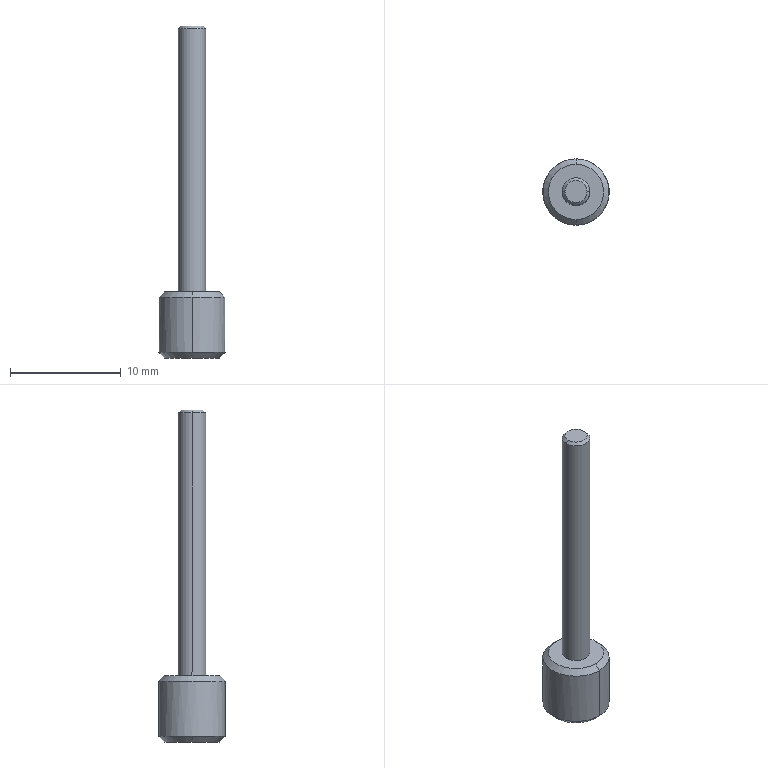Part | SolidWorks | features BaseBody 1 | 1 solid | 13 faces | box 6 x 6 x 30 mm | volume 282.776 mm3 | cone 6 | cylinder 4 | plane 3 | commonest cylinder face diameters 2.5 x2 6 x2
STEP:
#1=CARTESIAN_POINT('',(-45.25,9.997,38.261));
#2=VERTEX_POINT('',#1);
#3=CARTESIAN_POINT('',(-42.75,9.997,38.261));
#4=VERTEX_POINT('',#3);
#5=CARTESIAN_POINT('',(-44.,9.997,38.261));
#6=DIRECTION('',(0.,0.,-1.));
#7=DIRECTION('',(-1.,0.,0.));
#8=AXIS2_PLACEMENT_3D('',#5,#6,#7);
#9=CIRCLE('',#8,1.25);
#10=EDGE_CURVE('',#2,#4,#9,.T.);
#11=ORIENTED_EDGE('',*,*,#10,.T.);
#12=CARTESIAN_POINT('',(-42.75,9.997,14.511));
#13=VERTEX_POINT('',#12);
#14=CARTESIAN_POINT('',(-42.75,9.997,38.261));
#15=DIRECTION('',(0.,0.,-1.));
#16=VECTOR('',#15,1000.);
#17=LINE('',#14,#16);
#18=EDGE_CURVE('',#4,#13,#17,.T.);
#19=ORIENTED_EDGE('',*,*,#18,.T.);
#20=CARTESIAN_POINT('',(-45.25,9.997,14.511));
#21=VERTEX_POINT('',#20);
#22=CARTESIAN_POINT('',(-44.,9.997,14.511));
#23=DIRECTION('',(0.,0.,1.));
#24=DIRECTION('',(-1.,0.,0.));
#25=AXIS2_PLACEMENT_3D('',#22,#23,#24);
#26=CIRCLE('',#25,1.25);
#27=EDGE_CURVE('',#13,#21,#26,.T.);
#28=ORIENTED_EDGE('',*,*,#27,.T.);
#29=CARTESIAN_POINT('',(-45.25,9.997,38.261));
#30=DIRECTION('',(0.,0.,-1.));
#31=VECTOR('',#30,1000.);
#32=LINE('',#29,#31);
#33=EDGE_CURVE('',#2,#21,#32,.T.);
#34=ORIENTED_EDGE('',*,*,#33,.F.);
#35=EDGE_LOOP('',(#11,#19,#28,#34));
#36=FACE_OUTER_BOUND('',#35,.T.);
#37=CARTESIAN_POINT('',(-44.,9.997,38.261));
#38=DIRECTION('',(0.,0.,-1.));
#39=DIRECTION('',(-1.,0.,0.));
#40=AXIS2_PLACEMENT_3D('',#37,#38,#39);
#41=CYLINDRICAL_SURFACE('',#40,1.25);
#42=ADVANCED_FACE('',(#36),#41,.T.);
#43=CARTESIAN_POINT('',(-45.,9.997,38.511));
#44=VERTEX_POINT('',#43);
#45=CARTESIAN_POINT('',(-43.,9.997,38.511));
#46=VERTEX_POINT('',#45);
#47=CARTESIAN_POINT('',(-44.,9.997,38.511));
#48=DIRECTION('',(0.,0.,-1.));
#49=DIRECTION('',(-1.,0.,0.));
#50=AXIS2_PLACEMENT_3D('',#47,#48,#49);
#51=CIRCLE('',#50,1.);
#52=EDGE_CURVE('',#44,#46,#51,.T.);
#53=ORIENTED_EDGE('',*,*,#52,.T.);
#54=CARTESIAN_POINT('',(-42.75,9.997,38.261));
#55=DIRECTION('',(0.7071,0.,-0.7071));
#56=VECTOR('',#55,1000.);
#57=LINE('',#54,#56);
#58=EDGE_CURVE('',#46,#4,#57,.T.);
#59=ORIENTED_EDGE('',*,*,#58,.T.);
#60=ORIENTED_EDGE('',*,*,#10,.F.);
#61=CARTESIAN_POINT('',(-45.25,9.997,38.261));
#62=DIRECTION('',(-0.7071,0.,-0.7071));
#63=VECTOR('',#62,1000.);
#64=LINE('',#61,#63);
#65=EDGE_CURVE('',#44,#2,#64,.T.);
#66=ORIENTED_EDGE('',*,*,#65,.F.);
#67=EDGE_LOOP('',(#53,#59,#60,#66));
#68=FACE_OUTER_BOUND('',#67,.T.);
#69=CARTESIAN_POINT('',(-44.,9.997,38.261));
#70=DIRECTION('',(0.,0.,-1.));
#71=DIRECTION('',(-1.,0.,0.));
#72=AXIS2_PLACEMENT_3D('',#69,#70,#71);
#73=CONICAL_SURFACE('',#72,1.25,0.7854);
#74=ADVANCED_FACE('',(#68),#73,.T.);
#75=CARTESIAN_POINT('',(-44.,7.497,14.511));
#76=VERTEX_POINT('',#75);
#77=CARTESIAN_POINT('',(-44.,12.497,14.511));
#78=VERTEX_POINT('',#77);
#79=CARTESIAN_POINT('',(-44.,9.997,14.511));
#80=DIRECTION('',(0.,0.,1.));
#81=DIRECTION('',(0.,1.,0.));
#82=AXIS2_PLACEMENT_3D('',#79,#80,#81);
#83=CIRCLE('',#82,2.5);
#84=EDGE_CURVE('',#76,#78,#83,.T.);
#85=ORIENTED_EDGE('',*,*,#84,.F.);
#86=CARTESIAN_POINT('',(-44.,6.997,14.011));
#87=VERTEX_POINT('',#86);
#88=CARTESIAN_POINT('',(-44.,6.997,14.011));
#89=DIRECTION('',(0.,-0.7071,-0.7071));
#90=VECTOR('',#89,1000.);
#91=LINE('',#88,#90);
#92=EDGE_CURVE('',#76,#87,#91,.T.);
#93=ORIENTED_EDGE('',*,*,#92,.T.);
#94=CARTESIAN_POINT('',(-44.,12.997,14.011));
#95=VERTEX_POINT('',#94);
#96=CARTESIAN_POINT('',(-44.,9.997,14.011));
#97=DIRECTION('',(0.,0.,1.));
#98=DIRECTION('',(0.,1.,0.));
#99=AXIS2_PLACEMENT_3D('',#96,#97,#98);
#100=CIRCLE('',#99,3.);
#101=EDGE_CURVE('',#87,#95,#100,.T.);
#102=ORIENTED_EDGE('',*,*,#101,.T.);
#103=CARTESIAN_POINT('',(-44.,12.997,14.011));
#104=DIRECTION('',(0.,0.7071,-0.7071));
#105=VECTOR('',#104,1000.);
#106=LINE('',#103,#105);
#107=EDGE_CURVE('',#78,#95,#106,.T.);
#108=ORIENTED_EDGE('',*,*,#107,.F.);
#109=EDGE_LOOP('',(#85,#93,#102,#108));
#110=FACE_OUTER_BOUND('',#109,.T.);
#111=CARTESIAN_POINT('',(-44.,9.997,14.011));
#112=DIRECTION('',(0.,0.,-1.));
#113=DIRECTION('',(0.,1.,0.));
#114=AXIS2_PLACEMENT_3D('',#111,#112,#113);
#115=CONICAL_SURFACE('',#114,3.,0.7854);
#116=ADVANCED_FACE('',(#110),#115,.T.);
#117=ORIENTED_EDGE('',*,*,#101,.F.);
#118=CARTESIAN_POINT('',(-44.,6.997,9.011));
#119=VERTEX_POINT('',#118);
#120=CARTESIAN_POINT('',(-44.,6.997,14.011));
#121=DIRECTION('',(0.,0.,-1.));
#122=VECTOR('',#121,1000.);
#123=LINE('',#120,#122);
#124=EDGE_CURVE('',#87,#119,#123,.T.);
#125=ORIENTED_EDGE('',*,*,#124,.T.);
#126=CARTESIAN_POINT('',(-41.,9.997,9.011));
#127=VERTEX_POINT('',#126);
#128=CARTESIAN_POINT('',(-44.,9.997,9.011));
#129=DIRECTION('',(0.,0.,1.));
#130=DIRECTION('',(0.,1.,0.));
#131=AXIS2_PLACEMENT_3D('',#128,#129,#130);
#132=CIRCLE('',#131,3.);
#133=EDGE_CURVE('',#119,#127,#132,.T.);
#134=ORIENTED_EDGE('',*,*,#133,.T.);
#135=CARTESIAN_POINT('',(-44.,12.997,9.011));
#136=VERTEX_POINT('',#135);
#137=CARTESIAN_POINT('',(-44.,9.997,9.011));
#138=DIRECTION('',(0.,0.,1.));
#139=DIRECTION('',(0.,1.,0.));
#140=AXIS2_PLACEMENT_3D('',#137,#138,#139);
#141=CIRCLE('',#140,3.);
#142=EDGE_CURVE('',#127,#136,#141,.T.);
#143=ORIENTED_EDGE('',*,*,#142,.T.);
#144=CARTESIAN_POINT('',(-44.,12.997,14.011));
#145=DIRECTION('',(0.,0.,-1.));
#146=VECTOR('',#145,1000.);
#147=LINE('',#144,#146);
#148=EDGE_CURVE('',#95,#136,#147,.T.);
#149=ORIENTED_EDGE('',*,*,#148,.F.);
#150=EDGE_LOOP('',(#117,#125,#134,#143,#149));
#151=FACE_OUTER_BOUND('',#150,.T.);
#152=CARTESIAN_POINT('',(-44.,9.997,14.011));
#153=DIRECTION('',(0.,0.,-1.));
#154=DIRECTION('',(0.,1.,0.));
#155=AXIS2_PLACEMENT_3D('',#152,#153,#154);
#156=CYLINDRICAL_SURFACE('',#155,3.);
#157=ADVANCED_FACE('',(#151),#156,.T.);
#158=CARTESIAN_POINT('',(-41.5,9.997,8.511));
#159=VERTEX_POINT('',#158);
#160=CARTESIAN_POINT('',(-46.5,9.997,8.511));
#161=VERTEX_POINT('',#160);
#162=CARTESIAN_POINT('',(-44.,9.997,8.511));
#163=DIRECTION('',(0.,0.,1.));
#164=DIRECTION('',(1.,0.,0.));
#165=AXIS2_PLACEMENT_3D('',#162,#163,#164);
#166=CIRCLE('',#165,2.5);
#167=EDGE_CURVE('',#159,#161,#166,.T.);
#168=ORIENTED_EDGE('',*,*,#167,.T.);
#169=CARTESIAN_POINT('',(-47.,9.997,9.011));
#170=VERTEX_POINT('',#169);
#171=CARTESIAN_POINT('',(-47.,9.997,9.011));
#172=DIRECTION('',(-0.7071,0.,0.7071));
#173=VECTOR('',#172,1000.);
#174=LINE('',#171,#173);
#175=EDGE_CURVE('',#161,#170,#174,.T.);
#176=ORIENTED_EDGE('',*,*,#175,.T.);
#177=CARTESIAN_POINT('',(-44.,9.997,9.011));
#178=DIRECTION('',(0.,0.,1.));
#179=DIRECTION('',(0.,1.,0.));
#180=AXIS2_PLACEMENT_3D('',#177,#178,#179);
#181=CIRCLE('',#180,3.);
#182=EDGE_CURVE('',#136,#170,#181,.T.);
#183=ORIENTED_EDGE('',*,*,#182,.F.);
#184=ORIENTED_EDGE('',*,*,#142,.F.);
#185=CARTESIAN_POINT('',(-41.,9.997,9.011));
#186=DIRECTION('',(0.7071,0.,0.7071));
#187=VECTOR('',#186,1000.);
#188=LINE('',#185,#187);
#189=EDGE_CURVE('',#159,#127,#188,.T.);
#190=ORIENTED_EDGE('',*,*,#189,.F.);
#191=EDGE_LOOP('',(#168,#176,#183,#184,#190));
#192=FACE_OUTER_BOUND('',#191,.T.);
#193=CARTESIAN_POINT('',(-44.,9.997,9.011));
#194=DIRECTION('',(0.,0.,1.));
#195=DIRECTION('',(1.,0.,0.));
#196=AXIS2_PLACEMENT_3D('',#193,#194,#195);
#197=CONICAL_SURFACE('',#196,3.,0.7854);
#198=ADVANCED_FACE('',(#192),#197,.T.);
#199=ORIENTED_EDGE('',*,*,#18,.F.);
#200=CARTESIAN_POINT('',(-44.,9.997,38.261));
#201=DIRECTION('',(0.,0.,-1.));
#202=DIRECTION('',(-1.,0.,0.));
#203=AXIS2_PLACEMENT_3D('',#200,#201,#202);
#204=CIRCLE('',#203,1.25);
#205=EDGE_CURVE('',#4,#2,#204,.T.);
#206=ORIENTED_EDGE('',*,*,#205,.T.);
#207=ORIENTED_EDGE('',*,*,#33,.T.);
#208=CARTESIAN_POINT('',(-44.,9.997,14.511));
#209=DIRECTION('',(0.,0.,1.));
#210=DIRECTION('',(-1.,0.,0.));
#211=AXIS2_PLACEMENT_3D('',#208,#209,#210);
#212=CIRCLE('',#211,1.25);
#213=EDGE_CURVE('',#21,#13,#212,.T.);
#214=ORIENTED_EDGE('',*,*,#213,.T.);
#215=EDGE_LOOP('',(#199,#206,#207,#214));
#216=FACE_OUTER_BOUND('',#215,.T.);
#217=CARTESIAN_POINT('',(-44.,9.997,38.261));
#218=DIRECTION('',(0.,0.,-1.));
#219=DIRECTION('',(-1.,0.,0.));
#220=AXIS2_PLACEMENT_3D('',#217,#218,#219);
#221=CYLINDRICAL_SURFACE('',#220,1.25);
#222=ADVANCED_FACE('',(#216),#221,.T.);
#223=ORIENTED_EDGE('',*,*,#213,.F.);
#224=ORIENTED_EDGE('',*,*,#27,.F.);
#225=EDGE_LOOP('',(#223,#224));
#226=FACE_BOUND('',#225,.T.);
#227=CARTESIAN_POINT('',(-44.,9.997,14.511));
#228=DIRECTION('',(0.,0.,1.));
#229=DIRECTION('',(0.,1.,0.));
#230=AXIS2_PLACEMENT_3D('',#227,#228,#229);
#231=CIRCLE('',#230,2.5);
#232=EDGE_CURVE('',#78,#76,#231,.T.);
#233=ORIENTED_EDGE('',*,*,#232,.T.);
#234=ORIENTED_EDGE('',*,*,#84,.T.);
#235=EDGE_LOOP('',(#233,#234));
#236=FACE_OUTER_BOUND('',#235,.T.);
#237=CARTESIAN_POINT('',(-46.5,7.497,14.511));
#238=DIRECTION('',(0.,0.,1.));
#239=DIRECTION('',(1.,0.,0.));
#240=AXIS2_PLACEMENT_3D('',#237,#238,#239);
#241=PLANE('',#240);
#242=ADVANCED_FACE('',(#226,#236),#241,.T.);
#243=ORIENTED_EDGE('',*,*,#58,.F.);
#244=CARTESIAN_POINT('',(-44.,9.997,38.511));
#245=DIRECTION('',(0.,0.,-1.));
#246=DIRECTION('',(-1.,0.,0.));
#247=AXIS2_PLACEMENT_3D('',#244,#245,#246);
#248=CIRCLE('',#247,1.);
#249=EDGE_CURVE('',#46,#44,#248,.T.);
#250=ORIENTED_EDGE('',*,*,#249,.T.);
#251=ORIENTED_EDGE('',*,*,#65,.T.);
#252=ORIENTED_EDGE('',*,*,#205,.F.);
#253=EDGE_LOOP('',(#243,#250,#251,#252));
#254=FACE_OUTER_BOUND('',#253,.T.);
#255=CARTESIAN_POINT('',(-44.,9.997,38.261));
#256=DIRECTION('',(0.,0.,-1.));
#257=DIRECTION('',(-1.,0.,0.));
#258=AXIS2_PLACEMENT_3D('',#255,#256,#257);
#259=CONICAL_SURFACE('',#258,1.25,0.7854);
#260=ADVANCED_FACE('',(#254),#259,.T.);
#261=ORIENTED_EDGE('',*,*,#92,.F.);
#262=ORIENTED_EDGE('',*,*,#232,.F.);
#263=ORIENTED_EDGE('',*,*,#107,.T.);
#264=CARTESIAN_POINT('',(-44.,9.997,14.011));
#265=DIRECTION('',(0.,0.,1.));
#266=DIRECTION('',(0.,1.,0.));
#267=AXIS2_PLACEMENT_3D('',#264,#265,#266);
#268=CIRCLE('',#267,3.);
#269=EDGE_CURVE('',#95,#87,#268,.T.);
#270=ORIENTED_EDGE('',*,*,#269,.T.);
#271=EDGE_LOOP('',(#261,#262,#263,#270));
#272=FACE_OUTER_BOUND('',#271,.T.);
#273=CARTESIAN_POINT('',(-44.,9.997,14.011));
#274=DIRECTION('',(0.,0.,-1.));
#275=DIRECTION('',(0.,1.,0.));
#276=AXIS2_PLACEMENT_3D('',#273,#274,#275);
#277=CONICAL_SURFACE('',#276,3.,0.7854);
#278=ADVANCED_FACE('',(#272),#277,.T.);
#279=ORIENTED_EDGE('',*,*,#52,.F.);
#280=ORIENTED_EDGE('',*,*,#249,.F.);
#281=EDGE_LOOP('',(#279,#280));
#282=FACE_OUTER_BOUND('',#281,.T.);
#283=CARTESIAN_POINT('',(-45.,8.997,38.511));
#284=DIRECTION('',(0.,0.,1.));
#285=DIRECTION('',(1.,0.,0.));
#286=AXIS2_PLACEMENT_3D('',#283,#284,#285);
#287=PLANE('',#286);
#288=ADVANCED_FACE('',(#282),#287,.T.);
#289=ORIENTED_EDGE('',*,*,#124,.F.);
#290=ORIENTED_EDGE('',*,*,#269,.F.);
#291=ORIENTED_EDGE('',*,*,#148,.T.);
#292=ORIENTED_EDGE('',*,*,#182,.T.);
#293=CARTESIAN_POINT('',(-44.,9.997,9.011));
#294=DIRECTION('',(0.,0.,1.));
#295=DIRECTION('',(0.,1.,0.));
#296=AXIS2_PLACEMENT_3D('',#293,#294,#295);
#297=CIRCLE('',#296,3.);
#298=EDGE_CURVE('',#170,#119,#297,.T.);
#299=ORIENTED_EDGE('',*,*,#298,.T.);
#300=EDGE_LOOP('',(#289,#290,#291,#292,#299));
#301=FACE_OUTER_BOUND('',#300,.T.);
#302=CARTESIAN_POINT('',(-44.,9.997,14.011));
#303=DIRECTION('',(0.,0.,-1.));
#304=DIRECTION('',(0.,1.,0.));
#305=AXIS2_PLACEMENT_3D('',#302,#303,#304);
#306=CYLINDRICAL_SURFACE('',#305,3.);
#307=ADVANCED_FACE('',(#301),#306,.T.);
#308=ORIENTED_EDGE('',*,*,#175,.F.);
#309=CARTESIAN_POINT('',(-44.,9.997,8.511));
#310=DIRECTION('',(0.,0.,1.));
#311=DIRECTION('',(1.,0.,0.));
#312=AXIS2_PLACEMENT_3D('',#309,#310,#311);
#313=CIRCLE('',#312,2.5);
#314=EDGE_CURVE('',#161,#159,#313,.T.);
#315=ORIENTED_EDGE('',*,*,#314,.T.);
#316=ORIENTED_EDGE('',*,*,#189,.T.);
#317=ORIENTED_EDGE('',*,*,#133,.F.);
#318=ORIENTED_EDGE('',*,*,#298,.F.);
#319=EDGE_LOOP('',(#308,#315,#316,#317,#318));
#320=FACE_OUTER_BOUND('',#319,.T.);
#321=CARTESIAN_POINT('',(-44.,9.997,9.011));
#322=DIRECTION('',(0.,0.,1.));
#323=DIRECTION('',(1.,0.,0.));
#324=AXIS2_PLACEMENT_3D('',#321,#322,#323);
#325=CONICAL_SURFACE('',#324,3.,0.7854);
#326=ADVANCED_FACE('',(#320),#325,.T.);
#327=ORIENTED_EDGE('',*,*,#167,.F.);
#328=ORIENTED_EDGE('',*,*,#314,.F.);
#329=EDGE_LOOP('',(#327,#328));
#330=FACE_OUTER_BOUND('',#329,.T.);
#331=CARTESIAN_POINT('',(-46.5,7.497,8.511));
#332=DIRECTION('',(0.,0.,1.));
#333=DIRECTION('',(1.,0.,0.));
#334=AXIS2_PLACEMENT_3D('',#331,#332,#333);
#335=PLANE('',#334);
#336=ADVANCED_FACE('',(#330),#335,.F.);
#337=CLOSED_SHELL('',(#42,#74,#116,#157,#198,#222,#242,#260,#278,#288,#307,#326,#336));
#338=MANIFOLD_SOLID_BREP('',#337);
#339=CARTESIAN_POINT('',(0.,0.,0.));
#340=DIRECTION('',(0.,0.,1.));
#341=DIRECTION('',(1.,0.,0.));
#342=AXIS2_PLACEMENT_3D('',#339,#340,#341);
#343=(LENGTH_UNIT()NAMED_UNIT(*)SI_UNIT(.MILLI.,.METRE.));
#344=UNCERTAINTY_MEASURE_WITH_UNIT(LENGTH_MEASURE(0.00001),#343,'','');
#345=(NAMED_UNIT(*)PLANE_ANGLE_UNIT()SI_UNIT($,.RADIAN.));
#346=(NAMED_UNIT(*)SI_UNIT($,.STERADIAN.)SOLID_ANGLE_UNIT());
#347=(GEOMETRIC_REPRESENTATION_CONTEXT(3)GLOBAL_UNCERTAINTY_ASSIGNED_CONTEXT((#344))GLOBAL_UNIT_ASSIGNED_CONTEXT((#343,#345,#346))REPRESENTATION_CONTEXT('',''));
#348=ADVANCED_BREP_SHAPE_REPRESENTATION('',(#338,#342),#347);